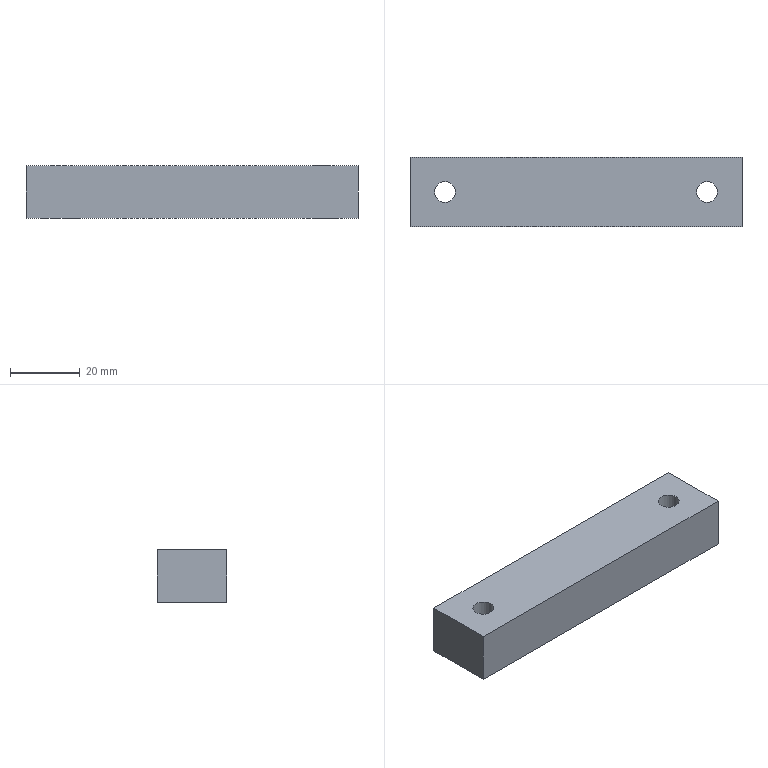Part | STEP file | gslz 2016.10.28-10_id2126_x_t | 1 solid | 12 faces | box 95 x 20 x 15 mm | volume 26584 mm3 | plane 8 | cylinder 4 | commonest cylinder face diameters 6 x2 11 x2
STEP:
#1=CARTESIAN_POINT('',(0.,0.,0.));
#2=DIRECTION('',(0.,0.,1.));
#3=DIRECTION('',(1.,0.,0.));
#4=AXIS2_PLACEMENT_3D('',#1,#2,#3);
#5=CARTESIAN_POINT('',(593.5,240.,28.));
#6=VERTEX_POINT('',#5);
#7=CARTESIAN_POINT('',(599.,240.,28.));
#8=DIRECTION('',(0.,0.,1.));
#9=DIRECTION('',(-1.,0.,0.));
#10=AXIS2_PLACEMENT_3D('',#7,#8,#9);
#11=CIRCLE('',#10,5.5);
#12=CARTESIAN_POINT('',(599.,240.,30.));
#13=DIRECTION('',(0.,0.,-1.));
#14=DIRECTION('',(-1.,0.,0.));
#15=AXIS2_PLACEMENT_3D('',#12,#13,#14);
#16=CYLINDRICAL_SURFACE('',#15,5.5);
#17=CARTESIAN_POINT('',(6.283,2.));
#18=DIRECTION('',(-1.,0.));
#19=VECTOR('',#18,1.);
#20=LINE('',#17,#19);
#21=(GEOMETRIC_REPRESENTATION_CONTEXT(2)PARAMETRIC_REPRESENTATION_CONTEXT()REPRESENTATION_CONTEXT('',''));
#22=DEFINITIONAL_REPRESENTATION('',(#20),#21);
#23=PCURVE('',#16,#22);
#24=CARTESIAN_POINT('',(636.5,240.,28.));
#25=DIRECTION('',(0.,0.,-1.));
#26=DIRECTION('',(1.,0.,0.));
#27=AXIS2_PLACEMENT_3D('',#24,#25,#26);
#28=PLANE('',#27);
#29=CARTESIAN_POINT('',(-43.,0.));
#30=CARTESIAN_POINT('',(-43.,9.526));
#31=CARTESIAN_POINT('',(-34.75,4.763));
#32=CARTESIAN_POINT('',(-26.5,0.));
#33=CARTESIAN_POINT('',(-34.75,-4.763));
#34=CARTESIAN_POINT('',(-43.,-9.526));
#35=CARTESIAN_POINT('',(-43.,0.));
#36=(BOUNDED_CURVE()B_SPLINE_CURVE(2,(#29,#30,#31,#32,#33,#34,#35),.UNSPECIFIED.,.T.,.F.)B_SPLINE_CURVE_WITH_KNOTS((1,2,2,2,2,1),(-2.094,0.,2.094,4.189,6.283,8.378),.UNSPECIFIED.)CURVE()GEOMETRIC_REPRESENTATION_ITEM()RATIONAL_B_SPLINE_CURVE((1.,0.5,1.,0.5,1.,0.5,1.))REPRESENTATION_ITEM(''));
#37=(GEOMETRIC_REPRESENTATION_CONTEXT(2)PARAMETRIC_REPRESENTATION_CONTEXT()REPRESENTATION_CONTEXT('',''));
#38=DEFINITIONAL_REPRESENTATION('',(#36),#37);
#39=PCURVE('',#28,#38);
#40=SURFACE_CURVE('',#11,(#23,#39),.PCURVE_S1.);
#41=EDGE_CURVE('',#6,#6,#40,.T.);
#42=ORIENTED_EDGE('',*,*,#41,.F.);
#43=CARTESIAN_POINT('',(593.5,240.,20.));
#44=VERTEX_POINT('',#43);
#45=CARTESIAN_POINT('',(593.5,240.,28.));
#46=CARTESIAN_POINT('',(593.5,240.,20.));
#47=B_SPLINE_CURVE_WITH_KNOTS('',1,(#45,#46),.UNSPECIFIED.,.F.,.F.,(2,2),(2.,10.),.PIECEWISE_BEZIER_KNOTS.);
#48=CARTESIAN_POINT('',(6.283,0.));
#49=DIRECTION('',(0.,1.));
#50=VECTOR('',#49,1.);
#51=LINE('',#48,#50);
#52=(GEOMETRIC_REPRESENTATION_CONTEXT(2)PARAMETRIC_REPRESENTATION_CONTEXT()REPRESENTATION_CONTEXT('',''));
#53=DEFINITIONAL_REPRESENTATION('',(#51),#52);
#54=PCURVE('',#16,#53);
#55=CARTESIAN_POINT('',(0.,0.));
#56=DIRECTION('',(0.,1.));
#57=VECTOR('',#56,1.);
#58=LINE('',#55,#57);
#59=(GEOMETRIC_REPRESENTATION_CONTEXT(2)PARAMETRIC_REPRESENTATION_CONTEXT()REPRESENTATION_CONTEXT('',''));
#60=DEFINITIONAL_REPRESENTATION('',(#58),#59);
#61=PCURVE('',#16,#60);
#62=SEAM_CURVE('',#47,(#54,#61),.PCURVE_S1.);
#63=EDGE_CURVE('',#6,#44,#62,.T.);
#64=ORIENTED_EDGE('',*,*,#63,.T.);
#65=CARTESIAN_POINT('',(604.5,240.,20.));
#66=VERTEX_POINT('',#65);
#67=CARTESIAN_POINT('',(599.,240.,20.));
#68=DIRECTION('',(0.,0.,1.));
#69=DIRECTION('',(1.,0.,0.));
#70=AXIS2_PLACEMENT_3D('',#67,#68,#69);
#71=CIRCLE('',#70,5.5);
#72=CARTESIAN_POINT('',(9.425,10.));
#73=DIRECTION('',(-1.,0.));
#74=VECTOR('',#73,1.);
#75=LINE('',#72,#74);
#76=(GEOMETRIC_REPRESENTATION_CONTEXT(2)PARAMETRIC_REPRESENTATION_CONTEXT()REPRESENTATION_CONTEXT('',''));
#77=DEFINITIONAL_REPRESENTATION('',(#75),#76);
#78=PCURVE('',#16,#77);
#79=CARTESIAN_POINT('',(581.5,240.,20.));
#80=DIRECTION('',(0.,0.,1.));
#81=DIRECTION('',(1.,0.,0.));
#82=AXIS2_PLACEMENT_3D('',#79,#80,#81);
#83=PLANE('',#82);
#84=CARTESIAN_POINT('',(17.5,0.));
#85=DIRECTION('',(1.,0.));
#86=AXIS2_PLACEMENT_2D('',#84,#85);
#87=CIRCLE('',#86,5.5);
#88=(GEOMETRIC_REPRESENTATION_CONTEXT(2)PARAMETRIC_REPRESENTATION_CONTEXT()REPRESENTATION_CONTEXT('',''));
#89=DEFINITIONAL_REPRESENTATION('',(#87),#88);
#90=PCURVE('',#83,#89);
#91=SURFACE_CURVE('',#71,(#78,#90),.PCURVE_S1.);
#92=EDGE_CURVE('',#44,#66,#91,.T.);
#93=ORIENTED_EDGE('',*,*,#92,.T.);
#94=CARTESIAN_POINT('',(599.,240.,20.));
#95=DIRECTION('',(0.,0.,1.));
#96=DIRECTION('',(1.,0.,0.));
#97=AXIS2_PLACEMENT_3D('',#94,#95,#96);
#98=CIRCLE('',#97,5.5);
#99=CARTESIAN_POINT('',(3.142,10.));
#100=DIRECTION('',(-1.,0.));
#101=VECTOR('',#100,1.);
#102=LINE('',#99,#101);
#103=(GEOMETRIC_REPRESENTATION_CONTEXT(2)PARAMETRIC_REPRESENTATION_CONTEXT()REPRESENTATION_CONTEXT('',''));
#104=DEFINITIONAL_REPRESENTATION('',(#102),#103);
#105=PCURVE('',#16,#104);
#106=CARTESIAN_POINT('',(17.5,0.));
#107=DIRECTION('',(1.,0.));
#108=AXIS2_PLACEMENT_2D('',#106,#107);
#109=CIRCLE('',#108,5.5);
#110=(GEOMETRIC_REPRESENTATION_CONTEXT(2)PARAMETRIC_REPRESENTATION_CONTEXT()REPRESENTATION_CONTEXT('',''));
#111=DEFINITIONAL_REPRESENTATION('',(#109),#110);
#112=PCURVE('',#83,#111);
#113=SURFACE_CURVE('',#98,(#105,#112),.PCURVE_S1.);
#114=EDGE_CURVE('',#66,#44,#113,.T.);
#115=ORIENTED_EDGE('',*,*,#114,.T.);
#116=ORIENTED_EDGE('',*,*,#63,.F.);
#117=EDGE_LOOP('',(#42,#64,#93,#115,#116));
#118=FACE_BOUND('',#117,.F.);
#119=ADVANCED_FACE('',(#118),#16,.F.);
#120=CARTESIAN_POINT('',(589.,250.,35.));
#121=VERTEX_POINT('',#120);
#122=CARTESIAN_POINT('',(589.,250.,20.));
#123=VERTEX_POINT('',#122);
#124=CARTESIAN_POINT('',(589.,250.,30.));
#125=DIRECTION('',(0.,0.,-1.));
#126=VECTOR('',#125,1.);
#127=LINE('',#124,#126);
#128=CARTESIAN_POINT('',(701.5,250.,30.));
#129=DIRECTION('',(0.,-1.,0.));
#130=DIRECTION('',(0.,0.,-1.));
#131=AXIS2_PLACEMENT_3D('',#128,#129,#130);
#132=PLANE('',#131);
#133=CARTESIAN_POINT('',(0.,-112.5));
#134=DIRECTION('',(1.,0.));
#135=VECTOR('',#134,1.);
#136=LINE('',#133,#135);
#137=(GEOMETRIC_REPRESENTATION_CONTEXT(2)PARAMETRIC_REPRESENTATION_CONTEXT()REPRESENTATION_CONTEXT('',''));
#138=DEFINITIONAL_REPRESENTATION('',(#136),#137);
#139=PCURVE('',#132,#138);
#140=CARTESIAN_POINT('',(589.,252.5,30.));
#141=DIRECTION('',(1.,0.,0.));
#142=DIRECTION('',(0.,0.,-1.));
#143=AXIS2_PLACEMENT_3D('',#140,#141,#142);
#144=PLANE('',#143);
#145=CARTESIAN_POINT('',(0.,-2.5));
#146=DIRECTION('',(1.,0.));
#147=VECTOR('',#146,1.);
#148=LINE('',#145,#147);
#149=(GEOMETRIC_REPRESENTATION_CONTEXT(2)PARAMETRIC_REPRESENTATION_CONTEXT()REPRESENTATION_CONTEXT('',''));
#150=DEFINITIONAL_REPRESENTATION('',(#148),#149);
#151=PCURVE('',#144,#150);
#152=SURFACE_CURVE('',#127,(#139,#151),.PCURVE_S1.);
#153=EDGE_CURVE('',#121,#123,#152,.T.);
#154=ORIENTED_EDGE('',*,*,#153,.F.);
#155=CARTESIAN_POINT('',(684.,250.,35.));
#156=VERTEX_POINT('',#155);
#157=CARTESIAN_POINT('',(581.5,250.,35.));
#158=DIRECTION('',(-1.,0.,0.));
#159=VECTOR('',#158,1.);
#160=LINE('',#157,#159);
#161=CARTESIAN_POINT('',(-5.,-120.));
#162=DIRECTION('',(0.,-1.));
#163=VECTOR('',#162,1.);
#164=LINE('',#161,#163);
#165=(GEOMETRIC_REPRESENTATION_CONTEXT(2)PARAMETRIC_REPRESENTATION_CONTEXT()REPRESENTATION_CONTEXT('',''));
#166=DEFINITIONAL_REPRESENTATION('',(#164),#165);
#167=PCURVE('',#132,#166);
#168=CARTESIAN_POINT('',(581.5,240.,35.));
#169=DIRECTION('',(0.,0.,1.));
#170=DIRECTION('',(1.,0.,0.));
#171=AXIS2_PLACEMENT_3D('',#168,#169,#170);
#172=PLANE('',#171);
#173=CARTESIAN_POINT('',(0.,10.));
#174=DIRECTION('',(-1.,0.));
#175=VECTOR('',#174,1.);
#176=LINE('',#173,#175);
#177=(GEOMETRIC_REPRESENTATION_CONTEXT(2)PARAMETRIC_REPRESENTATION_CONTEXT()REPRESENTATION_CONTEXT('',''));
#178=DEFINITIONAL_REPRESENTATION('',(#176),#177);
#179=PCURVE('',#172,#178);
#180=SURFACE_CURVE('',#160,(#167,#179),.PCURVE_S1.);
#181=EDGE_CURVE('',#156,#121,#180,.T.);
#182=ORIENTED_EDGE('',*,*,#181,.F.);
#183=CARTESIAN_POINT('',(684.,250.,20.));
#184=VERTEX_POINT('',#183);
#185=CARTESIAN_POINT('',(684.,250.,30.));
#186=DIRECTION('',(0.,0.,-1.));
#187=VECTOR('',#186,1.);
#188=LINE('',#185,#187);
#189=CARTESIAN_POINT('',(0.,-17.5));
#190=DIRECTION('',(1.,0.));
#191=VECTOR('',#190,1.);
#192=LINE('',#189,#191);
#193=(GEOMETRIC_REPRESENTATION_CONTEXT(2)PARAMETRIC_REPRESENTATION_CONTEXT()REPRESENTATION_CONTEXT('',''));
#194=DEFINITIONAL_REPRESENTATION('',(#192),#193);
#195=PCURVE('',#132,#194);
#196=CARTESIAN_POINT('',(684.,227.5,30.));
#197=DIRECTION('',(-1.,0.,0.));
#198=DIRECTION('',(0.,0.,1.));
#199=AXIS2_PLACEMENT_3D('',#196,#197,#198);
#200=PLANE('',#199);
#201=CARTESIAN_POINT('',(0.,22.5));
#202=DIRECTION('',(-1.,0.));
#203=VECTOR('',#202,1.);
#204=LINE('',#201,#203);
#205=(GEOMETRIC_REPRESENTATION_CONTEXT(2)PARAMETRIC_REPRESENTATION_CONTEXT()REPRESENTATION_CONTEXT('',''));
#206=DEFINITIONAL_REPRESENTATION('',(#204),#205);
#207=PCURVE('',#200,#206);
#208=SURFACE_CURVE('',#188,(#195,#207),.PCURVE_S1.);
#209=EDGE_CURVE('',#156,#184,#208,.T.);
#210=ORIENTED_EDGE('',*,*,#209,.T.);
#211=CARTESIAN_POINT('',(581.5,250.,20.));
#212=DIRECTION('',(-1.,0.,0.));
#213=VECTOR('',#212,1.);
#214=LINE('',#211,#213);
#215=CARTESIAN_POINT('',(10.,-120.));
#216=DIRECTION('',(0.,-1.));
#217=VECTOR('',#216,1.);
#218=LINE('',#215,#217);
#219=(GEOMETRIC_REPRESENTATION_CONTEXT(2)PARAMETRIC_REPRESENTATION_CONTEXT()REPRESENTATION_CONTEXT('',''));
#220=DEFINITIONAL_REPRESENTATION('',(#218),#219);
#221=PCURVE('',#132,#220);
#222=CARTESIAN_POINT('',(0.,10.));
#223=DIRECTION('',(-1.,0.));
#224=VECTOR('',#223,1.);
#225=LINE('',#222,#224);
#226=(GEOMETRIC_REPRESENTATION_CONTEXT(2)PARAMETRIC_REPRESENTATION_CONTEXT()REPRESENTATION_CONTEXT('',''));
#227=DEFINITIONAL_REPRESENTATION('',(#225),#226);
#228=PCURVE('',#83,#227);
#229=SURFACE_CURVE('',#214,(#221,#228),.PCURVE_S1.);
#230=EDGE_CURVE('',#184,#123,#229,.T.);
#231=ORIENTED_EDGE('',*,*,#230,.T.);
#232=EDGE_LOOP('',(#154,#182,#210,#231));
#233=FACE_BOUND('',#232,.T.);
#234=ADVANCED_FACE('',(#233),#132,.F.);
#235=ORIENTED_EDGE('',*,*,#209,.F.);
#236=CARTESIAN_POINT('',(684.,230.,35.));
#237=VERTEX_POINT('',#236);
#238=CARTESIAN_POINT('',(684.,227.5,35.));
#239=DIRECTION('',(0.,1.,0.));
#240=VECTOR('',#239,1.);
#241=LINE('',#238,#240);
#242=CARTESIAN_POINT('',(5.,0.));
#243=DIRECTION('',(0.,1.));
#244=VECTOR('',#243,1.);
#245=LINE('',#242,#244);
#246=(GEOMETRIC_REPRESENTATION_CONTEXT(2)PARAMETRIC_REPRESENTATION_CONTEXT()REPRESENTATION_CONTEXT('',''));
#247=DEFINITIONAL_REPRESENTATION('',(#245),#246);
#248=PCURVE('',#200,#247);
#249=CARTESIAN_POINT('',(102.5,-12.5));
#250=DIRECTION('',(0.,1.));
#251=VECTOR('',#250,1.);
#252=LINE('',#249,#251);
#253=(GEOMETRIC_REPRESENTATION_CONTEXT(2)PARAMETRIC_REPRESENTATION_CONTEXT()REPRESENTATION_CONTEXT('',''));
#254=DEFINITIONAL_REPRESENTATION('',(#252),#253);
#255=PCURVE('',#172,#254);
#256=SURFACE_CURVE('',#241,(#248,#255),.PCURVE_S1.);
#257=EDGE_CURVE('',#237,#156,#256,.T.);
#258=ORIENTED_EDGE('',*,*,#257,.F.);
#259=CARTESIAN_POINT('',(684.,230.,20.));
#260=VERTEX_POINT('',#259);
#261=CARTESIAN_POINT('',(684.,230.,30.));
#262=DIRECTION('',(0.,0.,-1.));
#263=VECTOR('',#262,1.);
#264=LINE('',#261,#263);
#265=CARTESIAN_POINT('',(0.,2.5));
#266=DIRECTION('',(-1.,0.));
#267=VECTOR('',#266,1.);
#268=LINE('',#265,#267);
#269=(GEOMETRIC_REPRESENTATION_CONTEXT(2)PARAMETRIC_REPRESENTATION_CONTEXT()REPRESENTATION_CONTEXT('',''));
#270=DEFINITIONAL_REPRESENTATION('',(#268),#269);
#271=PCURVE('',#200,#270);
#272=CARTESIAN_POINT('',(571.5,230.,30.));
#273=DIRECTION('',(0.,1.,0.));
#274=DIRECTION('',(0.,0.,1.));
#275=AXIS2_PLACEMENT_3D('',#272,#273,#274);
#276=PLANE('',#275);
#277=CARTESIAN_POINT('',(0.,112.5));
#278=DIRECTION('',(-1.,0.));
#279=VECTOR('',#278,1.);
#280=LINE('',#277,#279);
#281=(GEOMETRIC_REPRESENTATION_CONTEXT(2)PARAMETRIC_REPRESENTATION_CONTEXT()REPRESENTATION_CONTEXT('',''));
#282=DEFINITIONAL_REPRESENTATION('',(#280),#281);
#283=PCURVE('',#276,#282);
#284=SURFACE_CURVE('',#264,(#271,#283),.PCURVE_S1.);
#285=EDGE_CURVE('',#237,#260,#284,.T.);
#286=ORIENTED_EDGE('',*,*,#285,.T.);
#287=CARTESIAN_POINT('',(684.,227.5,20.));
#288=DIRECTION('',(0.,1.,0.));
#289=VECTOR('',#288,1.);
#290=LINE('',#287,#289);
#291=CARTESIAN_POINT('',(-10.,0.));
#292=DIRECTION('',(0.,1.));
#293=VECTOR('',#292,1.);
#294=LINE('',#291,#293);
#295=(GEOMETRIC_REPRESENTATION_CONTEXT(2)PARAMETRIC_REPRESENTATION_CONTEXT()REPRESENTATION_CONTEXT('',''));
#296=DEFINITIONAL_REPRESENTATION('',(#294),#295);
#297=PCURVE('',#200,#296);
#298=CARTESIAN_POINT('',(102.5,-12.5));
#299=DIRECTION('',(0.,1.));
#300=VECTOR('',#299,1.);
#301=LINE('',#298,#300);
#302=(GEOMETRIC_REPRESENTATION_CONTEXT(2)PARAMETRIC_REPRESENTATION_CONTEXT()REPRESENTATION_CONTEXT('',''));
#303=DEFINITIONAL_REPRESENTATION('',(#301),#302);
#304=PCURVE('',#83,#303);
#305=SURFACE_CURVE('',#290,(#297,#304),.PCURVE_S1.);
#306=EDGE_CURVE('',#260,#184,#305,.T.);
#307=ORIENTED_EDGE('',*,*,#306,.T.);
#308=EDGE_LOOP('',(#235,#258,#286,#307));
#309=FACE_BOUND('',#308,.T.);
#310=ADVANCED_FACE('',(#309),#200,.F.);
#311=ORIENTED_EDGE('',*,*,#285,.F.);
#312=CARTESIAN_POINT('',(589.,230.,35.));
#313=VERTEX_POINT('',#312);
#314=CARTESIAN_POINT('',(581.5,230.,35.));
#315=DIRECTION('',(1.,0.,0.));
#316=VECTOR('',#315,1.);
#317=LINE('',#314,#316);
#318=CARTESIAN_POINT('',(5.,10.));
#319=DIRECTION('',(0.,1.));
#320=VECTOR('',#319,1.);
#321=LINE('',#318,#320);
#322=(GEOMETRIC_REPRESENTATION_CONTEXT(2)PARAMETRIC_REPRESENTATION_CONTEXT()REPRESENTATION_CONTEXT('',''));
#323=DEFINITIONAL_REPRESENTATION('',(#321),#322);
#324=PCURVE('',#276,#323);
#325=CARTESIAN_POINT('',(0.,-10.));
#326=DIRECTION('',(1.,0.));
#327=VECTOR('',#326,1.);
#328=LINE('',#325,#327);
#329=(GEOMETRIC_REPRESENTATION_CONTEXT(2)PARAMETRIC_REPRESENTATION_CONTEXT()REPRESENTATION_CONTEXT('',''));
#330=DEFINITIONAL_REPRESENTATION('',(#328),#329);
#331=PCURVE('',#172,#330);
#332=SURFACE_CURVE('',#317,(#324,#331),.PCURVE_S1.);
#333=EDGE_CURVE('',#313,#237,#332,.T.);
#334=ORIENTED_EDGE('',*,*,#333,.F.);
#335=CARTESIAN_POINT('',(589.,230.,20.));
#336=VERTEX_POINT('',#335);
#337=CARTESIAN_POINT('',(589.,230.,30.));
#338=DIRECTION('',(0.,0.,-1.));
#339=VECTOR('',#338,1.);
#340=LINE('',#337,#339);
#341=CARTESIAN_POINT('',(0.,17.5));
#342=DIRECTION('',(-1.,0.));
#343=VECTOR('',#342,1.);
#344=LINE('',#341,#343);
#345=(GEOMETRIC_REPRESENTATION_CONTEXT(2)PARAMETRIC_REPRESENTATION_CONTEXT()REPRESENTATION_CONTEXT('',''));
#346=DEFINITIONAL_REPRESENTATION('',(#344),#345);
#347=PCURVE('',#276,#346);
#348=CARTESIAN_POINT('',(0.,-22.5));
#349=DIRECTION('',(1.,0.));
#350=VECTOR('',#349,1.);
#351=LINE('',#348,#350);
#352=(GEOMETRIC_REPRESENTATION_CONTEXT(2)PARAMETRIC_REPRESENTATION_CONTEXT()REPRESENTATION_CONTEXT('',''));
#353=DEFINITIONAL_REPRESENTATION('',(#351),#352);
#354=PCURVE('',#144,#353);
#355=SURFACE_CURVE('',#340,(#347,#354),.PCURVE_S1.);
#356=EDGE_CURVE('',#313,#336,#355,.T.);
#357=ORIENTED_EDGE('',*,*,#356,.T.);
#358=CARTESIAN_POINT('',(581.5,230.,20.));
#359=DIRECTION('',(1.,0.,0.));
#360=VECTOR('',#359,1.);
#361=LINE('',#358,#360);
#362=CARTESIAN_POINT('',(-10.,10.));
#363=DIRECTION('',(0.,1.));
#364=VECTOR('',#363,1.);
#365=LINE('',#362,#364);
#366=(GEOMETRIC_REPRESENTATION_CONTEXT(2)PARAMETRIC_REPRESENTATION_CONTEXT()REPRESENTATION_CONTEXT('',''));
#367=DEFINITIONAL_REPRESENTATION('',(#365),#366);
#368=PCURVE('',#276,#367);
#369=CARTESIAN_POINT('',(0.,-10.));
#370=DIRECTION('',(1.,0.));
#371=VECTOR('',#370,1.);
#372=LINE('',#369,#371);
#373=(GEOMETRIC_REPRESENTATION_CONTEXT(2)PARAMETRIC_REPRESENTATION_CONTEXT()REPRESENTATION_CONTEXT('',''));
#374=DEFINITIONAL_REPRESENTATION('',(#372),#373);
#375=PCURVE('',#83,#374);
#376=SURFACE_CURVE('',#361,(#368,#375),.PCURVE_S1.);
#377=EDGE_CURVE('',#336,#260,#376,.T.);
#378=ORIENTED_EDGE('',*,*,#377,.T.);
#379=EDGE_LOOP('',(#311,#334,#357,#378));
#380=FACE_BOUND('',#379,.T.);
#381=ADVANCED_FACE('',(#380),#276,.F.);
#382=ORIENTED_EDGE('',*,*,#356,.F.);
#383=CARTESIAN_POINT('',(589.,252.5,35.));
#384=DIRECTION('',(0.,-1.,0.));
#385=VECTOR('',#384,1.);
#386=LINE('',#383,#385);
#387=CARTESIAN_POINT('',(-5.,0.));
#388=DIRECTION('',(0.,-1.));
#389=VECTOR('',#388,1.);
#390=LINE('',#387,#389);
#391=(GEOMETRIC_REPRESENTATION_CONTEXT(2)PARAMETRIC_REPRESENTATION_CONTEXT()REPRESENTATION_CONTEXT('',''));
#392=DEFINITIONAL_REPRESENTATION('',(#390),#391);
#393=PCURVE('',#144,#392);
#394=CARTESIAN_POINT('',(7.5,12.5));
#395=DIRECTION('',(0.,-1.));
#396=VECTOR('',#395,1.);
#397=LINE('',#394,#396);
#398=(GEOMETRIC_REPRESENTATION_CONTEXT(2)PARAMETRIC_REPRESENTATION_CONTEXT()REPRESENTATION_CONTEXT('',''));
#399=DEFINITIONAL_REPRESENTATION('',(#397),#398);
#400=PCURVE('',#172,#399);
#401=SURFACE_CURVE('',#386,(#393,#400),.PCURVE_S1.);
#402=EDGE_CURVE('',#121,#313,#401,.T.);
#403=ORIENTED_EDGE('',*,*,#402,.F.);
#404=ORIENTED_EDGE('',*,*,#153,.T.);
#405=CARTESIAN_POINT('',(589.,252.5,20.));
#406=DIRECTION('',(0.,-1.,0.));
#407=VECTOR('',#406,1.);
#408=LINE('',#405,#407);
#409=CARTESIAN_POINT('',(10.,0.));
#410=DIRECTION('',(0.,-1.));
#411=VECTOR('',#410,1.);
#412=LINE('',#409,#411);
#413=(GEOMETRIC_REPRESENTATION_CONTEXT(2)PARAMETRIC_REPRESENTATION_CONTEXT()REPRESENTATION_CONTEXT('',''));
#414=DEFINITIONAL_REPRESENTATION('',(#412),#413);
#415=PCURVE('',#144,#414);
#416=CARTESIAN_POINT('',(7.5,12.5));
#417=DIRECTION('',(0.,-1.));
#418=VECTOR('',#417,1.);
#419=LINE('',#416,#418);
#420=(GEOMETRIC_REPRESENTATION_CONTEXT(2)PARAMETRIC_REPRESENTATION_CONTEXT()REPRESENTATION_CONTEXT('',''));
#421=DEFINITIONAL_REPRESENTATION('',(#419),#420);
#422=PCURVE('',#83,#421);
#423=SURFACE_CURVE('',#408,(#415,#422),.PCURVE_S1.);
#424=EDGE_CURVE('',#123,#336,#423,.T.);
#425=ORIENTED_EDGE('',*,*,#424,.T.);
#426=EDGE_LOOP('',(#382,#403,#404,#425));
#427=FACE_BOUND('',#426,.T.);
#428=ADVANCED_FACE('',(#427),#144,.F.);
#429=ORIENTED_EDGE('',*,*,#424,.F.);
#430=ORIENTED_EDGE('',*,*,#230,.F.);
#431=ORIENTED_EDGE('',*,*,#306,.F.);
#432=ORIENTED_EDGE('',*,*,#377,.F.);
#433=EDGE_LOOP('',(#429,#430,#431,#432));
#434=FACE_BOUND('',#433,.T.);
#435=ORIENTED_EDGE('',*,*,#114,.T.);
#436=ORIENTED_EDGE('',*,*,#92,.T.);
#437=EDGE_LOOP('',(#435,#436));
#438=FACE_BOUND('',#437,.T.);
#439=CARTESIAN_POINT('',(679.5,240.,20.));
#440=VERTEX_POINT('',#439);
#441=CARTESIAN_POINT('',(668.5,240.,20.));
#442=VERTEX_POINT('',#441);
#443=CARTESIAN_POINT('',(674.,240.,20.));
#444=DIRECTION('',(0.,0.,1.));
#445=DIRECTION('',(1.,0.,0.));
#446=AXIS2_PLACEMENT_3D('',#443,#444,#445);
#447=CIRCLE('',#446,5.5);
#448=CARTESIAN_POINT('',(92.5,0.));
#449=DIRECTION('',(1.,0.));
#450=AXIS2_PLACEMENT_2D('',#448,#449);
#451=CIRCLE('',#450,5.5);
#452=(GEOMETRIC_REPRESENTATION_CONTEXT(2)PARAMETRIC_REPRESENTATION_CONTEXT()REPRESENTATION_CONTEXT('',''));
#453=DEFINITIONAL_REPRESENTATION('',(#451),#452);
#454=PCURVE('',#83,#453);
#455=CARTESIAN_POINT('',(674.,240.,30.));
#456=DIRECTION('',(0.,0.,-1.));
#457=DIRECTION('',(-1.,0.,0.));
#458=AXIS2_PLACEMENT_3D('',#455,#456,#457);
#459=CYLINDRICAL_SURFACE('',#458,5.5);
#460=CARTESIAN_POINT('',(3.142,10.));
#461=DIRECTION('',(-1.,0.));
#462=VECTOR('',#461,1.);
#463=LINE('',#460,#462);
#464=(GEOMETRIC_REPRESENTATION_CONTEXT(2)PARAMETRIC_REPRESENTATION_CONTEXT()REPRESENTATION_CONTEXT('',''));
#465=DEFINITIONAL_REPRESENTATION('',(#463),#464);
#466=PCURVE('',#459,#465);
#467=SURFACE_CURVE('',#447,(#454,#466),.PCURVE_S1.);
#468=EDGE_CURVE('',#440,#442,#467,.T.);
#469=ORIENTED_EDGE('',*,*,#468,.T.);
#470=CARTESIAN_POINT('',(674.,240.,20.));
#471=DIRECTION('',(0.,0.,1.));
#472=DIRECTION('',(1.,0.,0.));
#473=AXIS2_PLACEMENT_3D('',#470,#471,#472);
#474=CIRCLE('',#473,5.5);
#475=CARTESIAN_POINT('',(92.5,0.));
#476=DIRECTION('',(1.,0.));
#477=AXIS2_PLACEMENT_2D('',#475,#476);
#478=CIRCLE('',#477,5.5);
#479=(GEOMETRIC_REPRESENTATION_CONTEXT(2)PARAMETRIC_REPRESENTATION_CONTEXT()REPRESENTATION_CONTEXT('',''));
#480=DEFINITIONAL_REPRESENTATION('',(#478),#479);
#481=PCURVE('',#83,#480);
#482=CARTESIAN_POINT('',(9.425,10.));
#483=DIRECTION('',(-1.,0.));
#484=VECTOR('',#483,1.);
#485=LINE('',#482,#484);
#486=(GEOMETRIC_REPRESENTATION_CONTEXT(2)PARAMETRIC_REPRESENTATION_CONTEXT()REPRESENTATION_CONTEXT('',''));
#487=DEFINITIONAL_REPRESENTATION('',(#485),#486);
#488=PCURVE('',#459,#487);
#489=SURFACE_CURVE('',#474,(#481,#488),.PCURVE_S1.);
#490=EDGE_CURVE('',#442,#440,#489,.T.);
#491=ORIENTED_EDGE('',*,*,#490,.T.);
#492=EDGE_LOOP('',(#469,#491));
#493=FACE_BOUND('',#492,.T.);
#494=ADVANCED_FACE('',(#434,#438,#493),#83,.F.);
#495=CARTESIAN_POINT('',(668.5,240.,28.));
#496=VERTEX_POINT('',#495);
#497=CARTESIAN_POINT('',(674.,240.,28.));
#498=DIRECTION('',(0.,0.,1.));
#499=DIRECTION('',(-1.,0.,0.));
#500=AXIS2_PLACEMENT_3D('',#497,#498,#499);
#501=CIRCLE('',#500,5.5);
#502=CARTESIAN_POINT('',(6.283,2.));
#503=DIRECTION('',(-1.,0.));
#504=VECTOR('',#503,1.);
#505=LINE('',#502,#504);
#506=(GEOMETRIC_REPRESENTATION_CONTEXT(2)PARAMETRIC_REPRESENTATION_CONTEXT()REPRESENTATION_CONTEXT('',''));
#507=DEFINITIONAL_REPRESENTATION('',(#505),#506);
#508=PCURVE('',#459,#507);
#509=CARTESIAN_POINT('',(636.5,240.,28.));
#510=DIRECTION('',(0.,0.,-1.));
#511=DIRECTION('',(1.,0.,0.));
#512=AXIS2_PLACEMENT_3D('',#509,#510,#511);
#513=PLANE('',#512);
#514=CARTESIAN_POINT('',(32.,0.));
#515=CARTESIAN_POINT('',(32.,9.526));
#516=CARTESIAN_POINT('',(40.25,4.763));
#517=CARTESIAN_POINT('',(48.5,0.));
#518=CARTESIAN_POINT('',(40.25,-4.763));
#519=CARTESIAN_POINT('',(32.,-9.526));
#520=CARTESIAN_POINT('',(32.,0.));
#521=(BOUNDED_CURVE()B_SPLINE_CURVE(2,(#514,#515,#516,#517,#518,#519,#520),.UNSPECIFIED.,.T.,.F.)B_SPLINE_CURVE_WITH_KNOTS((1,2,2,2,2,1),(-2.094,0.,2.094,4.189,6.283,8.378),.UNSPECIFIED.)CURVE()GEOMETRIC_REPRESENTATION_ITEM()RATIONAL_B_SPLINE_CURVE((1.,0.5,1.,0.5,1.,0.5,1.))REPRESENTATION_ITEM(''));
#522=(GEOMETRIC_REPRESENTATION_CONTEXT(2)PARAMETRIC_REPRESENTATION_CONTEXT()REPRESENTATION_CONTEXT('',''));
#523=DEFINITIONAL_REPRESENTATION('',(#521),#522);
#524=PCURVE('',#513,#523);
#525=SURFACE_CURVE('',#501,(#508,#524),.PCURVE_S1.);
#526=EDGE_CURVE('',#496,#496,#525,.T.);
#527=ORIENTED_EDGE('',*,*,#526,.F.);
#528=CARTESIAN_POINT('',(668.5,240.,28.));
#529=CARTESIAN_POINT('',(668.5,240.,20.));
#530=B_SPLINE_CURVE_WITH_KNOTS('',1,(#528,#529),.UNSPECIFIED.,.F.,.F.,(2,2),(2.,10.),.PIECEWISE_BEZIER_KNOTS.);
#531=CARTESIAN_POINT('',(6.283,0.));
#532=DIRECTION('',(0.,1.));
#533=VECTOR('',#532,1.);
#534=LINE('',#531,#533);
#535=(GEOMETRIC_REPRESENTATION_CONTEXT(2)PARAMETRIC_REPRESENTATION_CONTEXT()REPRESENTATION_CONTEXT('',''));
#536=DEFINITIONAL_REPRESENTATION('',(#534),#535);
#537=PCURVE('',#459,#536);
#538=CARTESIAN_POINT('',(0.,0.));
#539=DIRECTION('',(0.,1.));
#540=VECTOR('',#539,1.);
#541=LINE('',#538,#540);
#542=(GEOMETRIC_REPRESENTATION_CONTEXT(2)PARAMETRIC_REPRESENTATION_CONTEXT()REPRESENTATION_CONTEXT('',''));
#543=DEFINITIONAL_REPRESENTATION('',(#541),#542);
#544=PCURVE('',#459,#543);
#545=SEAM_CURVE('',#530,(#537,#544),.PCURVE_S1.);
#546=EDGE_CURVE('',#496,#442,#545,.T.);
#547=ORIENTED_EDGE('',*,*,#546,.T.);
#548=ORIENTED_EDGE('',*,*,#490,.T.);
#549=ORIENTED_EDGE('',*,*,#468,.T.);
#550=ORIENTED_EDGE('',*,*,#546,.F.);
#551=EDGE_LOOP('',(#527,#547,#548,#549,#550));
#552=FACE_BOUND('',#551,.F.);
#553=ADVANCED_FACE('',(#552),#459,.F.);
#554=CARTESIAN_POINT('',(671.,240.,28.));
#555=VERTEX_POINT('',#554);
#556=CARTESIAN_POINT('',(674.,240.,28.));
#557=DIRECTION('',(0.,0.,-1.));
#558=DIRECTION('',(-1.,0.,0.));
#559=AXIS2_PLACEMENT_3D('',#556,#557,#558);
#560=CIRCLE('',#559,3.);
#561=CARTESIAN_POINT('',(37.5,0.));
#562=DIRECTION('',(-1.,0.));
#563=AXIS2_PLACEMENT_2D('',#561,#562);
#564=CIRCLE('',#563,3.);
#565=(GEOMETRIC_REPRESENTATION_CONTEXT(2)PARAMETRIC_REPRESENTATION_CONTEXT()REPRESENTATION_CONTEXT('',''));
#566=DEFINITIONAL_REPRESENTATION('',(#564),#565);
#567=PCURVE('',#513,#566);
#568=CARTESIAN_POINT('',(674.,240.,30.));
#569=DIRECTION('',(0.,0.,-1.));
#570=DIRECTION('',(-1.,0.,0.));
#571=AXIS2_PLACEMENT_3D('',#568,#569,#570);
#572=CYLINDRICAL_SURFACE('',#571,3.);
#573=CARTESIAN_POINT('',(0.,2.));
#574=DIRECTION('',(1.,0.));
#575=VECTOR('',#574,1.);
#576=LINE('',#573,#575);
#577=(GEOMETRIC_REPRESENTATION_CONTEXT(2)PARAMETRIC_REPRESENTATION_CONTEXT()REPRESENTATION_CONTEXT('',''));
#578=DEFINITIONAL_REPRESENTATION('',(#576),#577);
#579=PCURVE('',#572,#578);
#580=SURFACE_CURVE('',#560,(#567,#579),.PCURVE_S1.);
#581=EDGE_CURVE('',#555,#555,#580,.T.);
#582=ORIENTED_EDGE('',*,*,#581,.F.);
#583=EDGE_LOOP('',(#582));
#584=FACE_BOUND('',#583,.T.);
#585=ORIENTED_EDGE('',*,*,#526,.F.);
#586=EDGE_LOOP('',(#585));
#587=FACE_BOUND('',#586,.T.);
#588=ADVANCED_FACE('',(#584,#587),#513,.T.);
#589=CARTESIAN_POINT('',(596.,240.,28.));
#590=VERTEX_POINT('',#589);
#591=CARTESIAN_POINT('',(599.,240.,28.));
#592=DIRECTION('',(0.,0.,-1.));
#593=DIRECTION('',(-1.,0.,0.));
#594=AXIS2_PLACEMENT_3D('',#591,#592,#593);
#595=CIRCLE('',#594,3.);
#596=CARTESIAN_POINT('',(-37.5,0.));
#597=DIRECTION('',(-1.,0.));
#598=AXIS2_PLACEMENT_2D('',#596,#597);
#599=CIRCLE('',#598,3.);
#600=(GEOMETRIC_REPRESENTATION_CONTEXT(2)PARAMETRIC_REPRESENTATION_CONTEXT()REPRESENTATION_CONTEXT('',''));
#601=DEFINITIONAL_REPRESENTATION('',(#599),#600);
#602=PCURVE('',#28,#601);
#603=CARTESIAN_POINT('',(599.,240.,30.));
#604=DIRECTION('',(0.,0.,-1.));
#605=DIRECTION('',(-1.,0.,0.));
#606=AXIS2_PLACEMENT_3D('',#603,#604,#605);
#607=CYLINDRICAL_SURFACE('',#606,3.);
#608=CARTESIAN_POINT('',(0.,2.));
#609=DIRECTION('',(1.,0.));
#610=VECTOR('',#609,1.);
#611=LINE('',#608,#610);
#612=(GEOMETRIC_REPRESENTATION_CONTEXT(2)PARAMETRIC_REPRESENTATION_CONTEXT()REPRESENTATION_CONTEXT('',''));
#613=DEFINITIONAL_REPRESENTATION('',(#611),#612);
#614=PCURVE('',#607,#613);
#615=SURFACE_CURVE('',#595,(#602,#614),.PCURVE_S1.);
#616=EDGE_CURVE('',#590,#590,#615,.T.);
#617=ORIENTED_EDGE('',*,*,#616,.F.);
#618=EDGE_LOOP('',(#617));
#619=FACE_BOUND('',#618,.T.);
#620=ORIENTED_EDGE('',*,*,#41,.F.);
#621=EDGE_LOOP('',(#620));
#622=FACE_BOUND('',#621,.T.);
#623=ADVANCED_FACE('',(#619,#622),#28,.T.);
#624=CARTESIAN_POINT('',(596.,240.,35.));
#625=VERTEX_POINT('',#624);
#626=CARTESIAN_POINT('',(602.,240.,35.));
#627=VERTEX_POINT('',#626);
#628=CARTESIAN_POINT('',(599.,240.,35.));
#629=DIRECTION('',(0.,0.,1.));
#630=DIRECTION('',(1.,0.,0.));
#631=AXIS2_PLACEMENT_3D('',#628,#629,#630);
#632=CIRCLE('',#631,3.);
#633=CARTESIAN_POINT('',(9.425,-5.));
#634=DIRECTION('',(-1.,0.));
#635=VECTOR('',#634,1.);
#636=LINE('',#633,#635);
#637=(GEOMETRIC_REPRESENTATION_CONTEXT(2)PARAMETRIC_REPRESENTATION_CONTEXT()REPRESENTATION_CONTEXT('',''));
#638=DEFINITIONAL_REPRESENTATION('',(#636),#637);
#639=PCURVE('',#607,#638);
#640=CARTESIAN_POINT('',(17.5,0.));
#641=DIRECTION('',(1.,0.));
#642=AXIS2_PLACEMENT_2D('',#640,#641);
#643=CIRCLE('',#642,3.);
#644=(GEOMETRIC_REPRESENTATION_CONTEXT(2)PARAMETRIC_REPRESENTATION_CONTEXT()REPRESENTATION_CONTEXT('',''));
#645=DEFINITIONAL_REPRESENTATION('',(#643),#644);
#646=PCURVE('',#172,#645);
#647=SURFACE_CURVE('',#632,(#639,#646),.PCURVE_S1.);
#648=EDGE_CURVE('',#625,#627,#647,.T.);
#649=ORIENTED_EDGE('',*,*,#648,.F.);
#650=CARTESIAN_POINT('',(596.,240.,35.));
#651=CARTESIAN_POINT('',(596.,240.,28.));
#652=B_SPLINE_CURVE_WITH_KNOTS('',1,(#650,#651),.UNSPECIFIED.,.F.,.F.,(2,2),(-5.,2.),.PIECEWISE_BEZIER_KNOTS.);
#653=CARTESIAN_POINT('',(6.283,0.));
#654=DIRECTION('',(0.,1.));
#655=VECTOR('',#654,1.);
#656=LINE('',#653,#655);
#657=(GEOMETRIC_REPRESENTATION_CONTEXT(2)PARAMETRIC_REPRESENTATION_CONTEXT()REPRESENTATION_CONTEXT('',''));
#658=DEFINITIONAL_REPRESENTATION('',(#656),#657);
#659=PCURVE('',#607,#658);
#660=CARTESIAN_POINT('',(0.,0.));
#661=DIRECTION('',(0.,1.));
#662=VECTOR('',#661,1.);
#663=LINE('',#660,#662);
#664=(GEOMETRIC_REPRESENTATION_CONTEXT(2)PARAMETRIC_REPRESENTATION_CONTEXT()REPRESENTATION_CONTEXT('',''));
#665=DEFINITIONAL_REPRESENTATION('',(#663),#664);
#666=PCURVE('',#607,#665);
#667=SEAM_CURVE('',#652,(#659,#666),.PCURVE_S1.);
#668=EDGE_CURVE('',#625,#590,#667,.T.);
#669=ORIENTED_EDGE('',*,*,#668,.T.);
#670=ORIENTED_EDGE('',*,*,#616,.F.);
#671=ORIENTED_EDGE('',*,*,#668,.F.);
#672=CARTESIAN_POINT('',(599.,240.,35.));
#673=DIRECTION('',(0.,0.,1.));
#674=DIRECTION('',(1.,0.,0.));
#675=AXIS2_PLACEMENT_3D('',#672,#673,#674);
#676=CIRCLE('',#675,3.);
#677=CARTESIAN_POINT('',(3.142,-5.));
#678=DIRECTION('',(-1.,0.));
#679=VECTOR('',#678,1.);
#680=LINE('',#677,#679);
#681=(GEOMETRIC_REPRESENTATION_CONTEXT(2)PARAMETRIC_REPRESENTATION_CONTEXT()REPRESENTATION_CONTEXT('',''));
#682=DEFINITIONAL_REPRESENTATION('',(#680),#681);
#683=PCURVE('',#607,#682);
#684=CARTESIAN_POINT('',(17.5,0.));
#685=DIRECTION('',(1.,0.));
#686=AXIS2_PLACEMENT_2D('',#684,#685);
#687=CIRCLE('',#686,3.);
#688=(GEOMETRIC_REPRESENTATION_CONTEXT(2)PARAMETRIC_REPRESENTATION_CONTEXT()REPRESENTATION_CONTEXT('',''));
#689=DEFINITIONAL_REPRESENTATION('',(#687),#688);
#690=PCURVE('',#172,#689);
#691=SURFACE_CURVE('',#676,(#683,#690),.PCURVE_S1.);
#692=EDGE_CURVE('',#627,#625,#691,.T.);
#693=ORIENTED_EDGE('',*,*,#692,.F.);
#694=EDGE_LOOP('',(#649,#669,#670,#671,#693));
#695=FACE_BOUND('',#694,.F.);
#696=ADVANCED_FACE('',(#695),#607,.F.);
#697=CARTESIAN_POINT('',(671.,240.,35.));
#698=VERTEX_POINT('',#697);
#699=CARTESIAN_POINT('',(677.,240.,35.));
#700=VERTEX_POINT('',#699);
#701=CARTESIAN_POINT('',(674.,240.,35.));
#702=DIRECTION('',(0.,0.,1.));
#703=DIRECTION('',(1.,0.,0.));
#704=AXIS2_PLACEMENT_3D('',#701,#702,#703);
#705=CIRCLE('',#704,3.);
#706=CARTESIAN_POINT('',(9.425,-5.));
#707=DIRECTION('',(-1.,0.));
#708=VECTOR('',#707,1.);
#709=LINE('',#706,#708);
#710=(GEOMETRIC_REPRESENTATION_CONTEXT(2)PARAMETRIC_REPRESENTATION_CONTEXT()REPRESENTATION_CONTEXT('',''));
#711=DEFINITIONAL_REPRESENTATION('',(#709),#710);
#712=PCURVE('',#572,#711);
#713=CARTESIAN_POINT('',(92.5,0.));
#714=DIRECTION('',(1.,0.));
#715=AXIS2_PLACEMENT_2D('',#713,#714);
#716=CIRCLE('',#715,3.);
#717=(GEOMETRIC_REPRESENTATION_CONTEXT(2)PARAMETRIC_REPRESENTATION_CONTEXT()REPRESENTATION_CONTEXT('',''));
#718=DEFINITIONAL_REPRESENTATION('',(#716),#717);
#719=PCURVE('',#172,#718);
#720=SURFACE_CURVE('',#705,(#712,#719),.PCURVE_S1.);
#721=EDGE_CURVE('',#698,#700,#720,.T.);
#722=ORIENTED_EDGE('',*,*,#721,.F.);
#723=CARTESIAN_POINT('',(671.,240.,35.));
#724=CARTESIAN_POINT('',(671.,240.,28.));
#725=B_SPLINE_CURVE_WITH_KNOTS('',1,(#723,#724),.UNSPECIFIED.,.F.,.F.,(2,2),(-5.,2.),.PIECEWISE_BEZIER_KNOTS.);
#726=CARTESIAN_POINT('',(6.283,0.));
#727=DIRECTION('',(0.,1.));
#728=VECTOR('',#727,1.);
#729=LINE('',#726,#728);
#730=(GEOMETRIC_REPRESENTATION_CONTEXT(2)PARAMETRIC_REPRESENTATION_CONTEXT()REPRESENTATION_CONTEXT('',''));
#731=DEFINITIONAL_REPRESENTATION('',(#729),#730);
#732=PCURVE('',#572,#731);
#733=CARTESIAN_POINT('',(0.,0.));
#734=DIRECTION('',(0.,1.));
#735=VECTOR('',#734,1.);
#736=LINE('',#733,#735);
#737=(GEOMETRIC_REPRESENTATION_CONTEXT(2)PARAMETRIC_REPRESENTATION_CONTEXT()REPRESENTATION_CONTEXT('',''));
#738=DEFINITIONAL_REPRESENTATION('',(#736),#737);
#739=PCURVE('',#572,#738);
#740=SEAM_CURVE('',#725,(#732,#739),.PCURVE_S1.);
#741=EDGE_CURVE('',#698,#555,#740,.T.);
#742=ORIENTED_EDGE('',*,*,#741,.T.);
#743=ORIENTED_EDGE('',*,*,#581,.F.);
#744=ORIENTED_EDGE('',*,*,#741,.F.);
#745=CARTESIAN_POINT('',(674.,240.,35.));
#746=DIRECTION('',(0.,0.,1.));
#747=DIRECTION('',(1.,0.,0.));
#748=AXIS2_PLACEMENT_3D('',#745,#746,#747);
#749=CIRCLE('',#748,3.);
#750=CARTESIAN_POINT('',(3.142,-5.));
#751=DIRECTION('',(-1.,0.));
#752=VECTOR('',#751,1.);
#753=LINE('',#750,#752);
#754=(GEOMETRIC_REPRESENTATION_CONTEXT(2)PARAMETRIC_REPRESENTATION_CONTEXT()REPRESENTATION_CONTEXT('',''));
#755=DEFINITIONAL_REPRESENTATION('',(#753),#754);
#756=PCURVE('',#572,#755);
#757=CARTESIAN_POINT('',(92.5,0.));
#758=DIRECTION('',(1.,0.));
#759=AXIS2_PLACEMENT_2D('',#757,#758);
#760=CIRCLE('',#759,3.);
#761=(GEOMETRIC_REPRESENTATION_CONTEXT(2)PARAMETRIC_REPRESENTATION_CONTEXT()REPRESENTATION_CONTEXT('',''));
#762=DEFINITIONAL_REPRESENTATION('',(#760),#761);
#763=PCURVE('',#172,#762);
#764=SURFACE_CURVE('',#749,(#756,#763),.PCURVE_S1.);
#765=EDGE_CURVE('',#700,#698,#764,.T.);
#766=ORIENTED_EDGE('',*,*,#765,.F.);
#767=EDGE_LOOP('',(#722,#742,#743,#744,#766));
#768=FACE_BOUND('',#767,.F.);
#769=ADVANCED_FACE('',(#768),#572,.F.);
#770=ORIENTED_EDGE('',*,*,#402,.T.);
#771=ORIENTED_EDGE('',*,*,#333,.T.);
#772=ORIENTED_EDGE('',*,*,#257,.T.);
#773=ORIENTED_EDGE('',*,*,#181,.T.);
#774=EDGE_LOOP('',(#770,#771,#772,#773));
#775=FACE_BOUND('',#774,.T.);
#776=ORIENTED_EDGE('',*,*,#692,.F.);
#777=ORIENTED_EDGE('',*,*,#648,.F.);
#778=EDGE_LOOP('',(#776,#777));
#779=FACE_BOUND('',#778,.T.);
#780=ORIENTED_EDGE('',*,*,#765,.F.);
#781=ORIENTED_EDGE('',*,*,#721,.F.);
#782=EDGE_LOOP('',(#780,#781));
#783=FACE_BOUND('',#782,.T.);
#784=ADVANCED_FACE('',(#775,#779,#783),#172,.T.);
#785=CLOSED_SHELL('',(#119,#234,#310,#381,#428,#494,#553,#588,#623,#696,#769,#784));
#786=MANIFOLD_SOLID_BREP('',#785);
#787=(LENGTH_UNIT()NAMED_UNIT(*)SI_UNIT(.MILLI.,.METRE.));
#788=UNCERTAINTY_MEASURE_WITH_UNIT(LENGTH_MEASURE(0.000002),#787,'','');
#789=(NAMED_UNIT(*)PLANE_ANGLE_UNIT()SI_UNIT($,.RADIAN.));
#790=(NAMED_UNIT(*)SI_UNIT($,.STERADIAN.)SOLID_ANGLE_UNIT());
#791=(GEOMETRIC_REPRESENTATION_CONTEXT(3)GLOBAL_UNCERTAINTY_ASSIGNED_CONTEXT((#788))GLOBAL_UNIT_ASSIGNED_CONTEXT((#787,#789,#790))REPRESENTATION_CONTEXT('',''));
#792=ADVANCED_BREP_SHAPE_REPRESENTATION('',(#4,#786),#791);